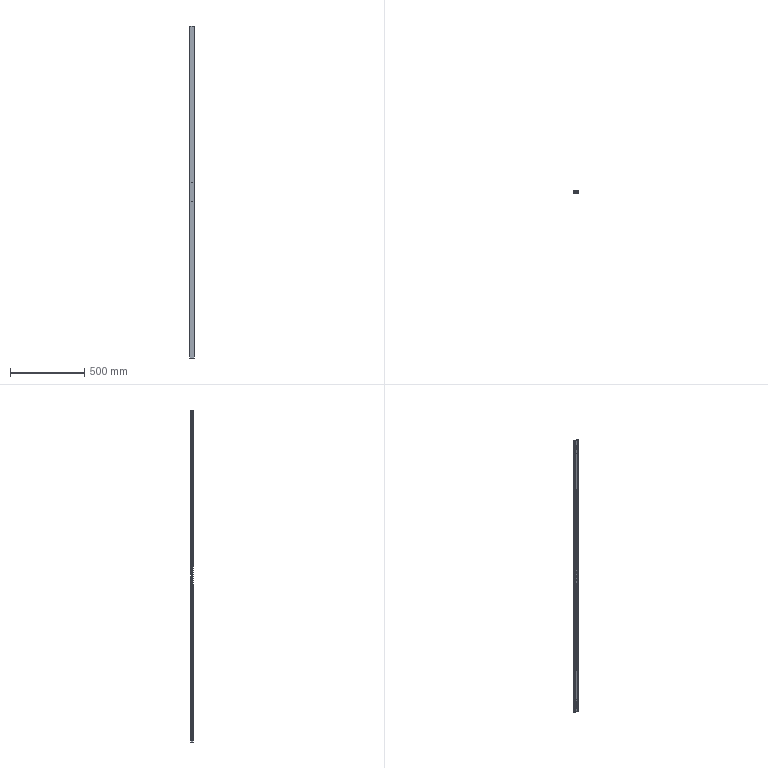Part | SolidWorks | features HoleWzd 3, BaseBody 1, MoveFace 1 | 1 solid | 176 faces | box 30 x 15 x 2236 mm | volume 538276 mm3 | cylinder 88 | plane 72 | cone 16 | commonest cylinder face diameters 5 x26 3.3 x24 4.5 x16 1 x12 2 x4 6.6 x4